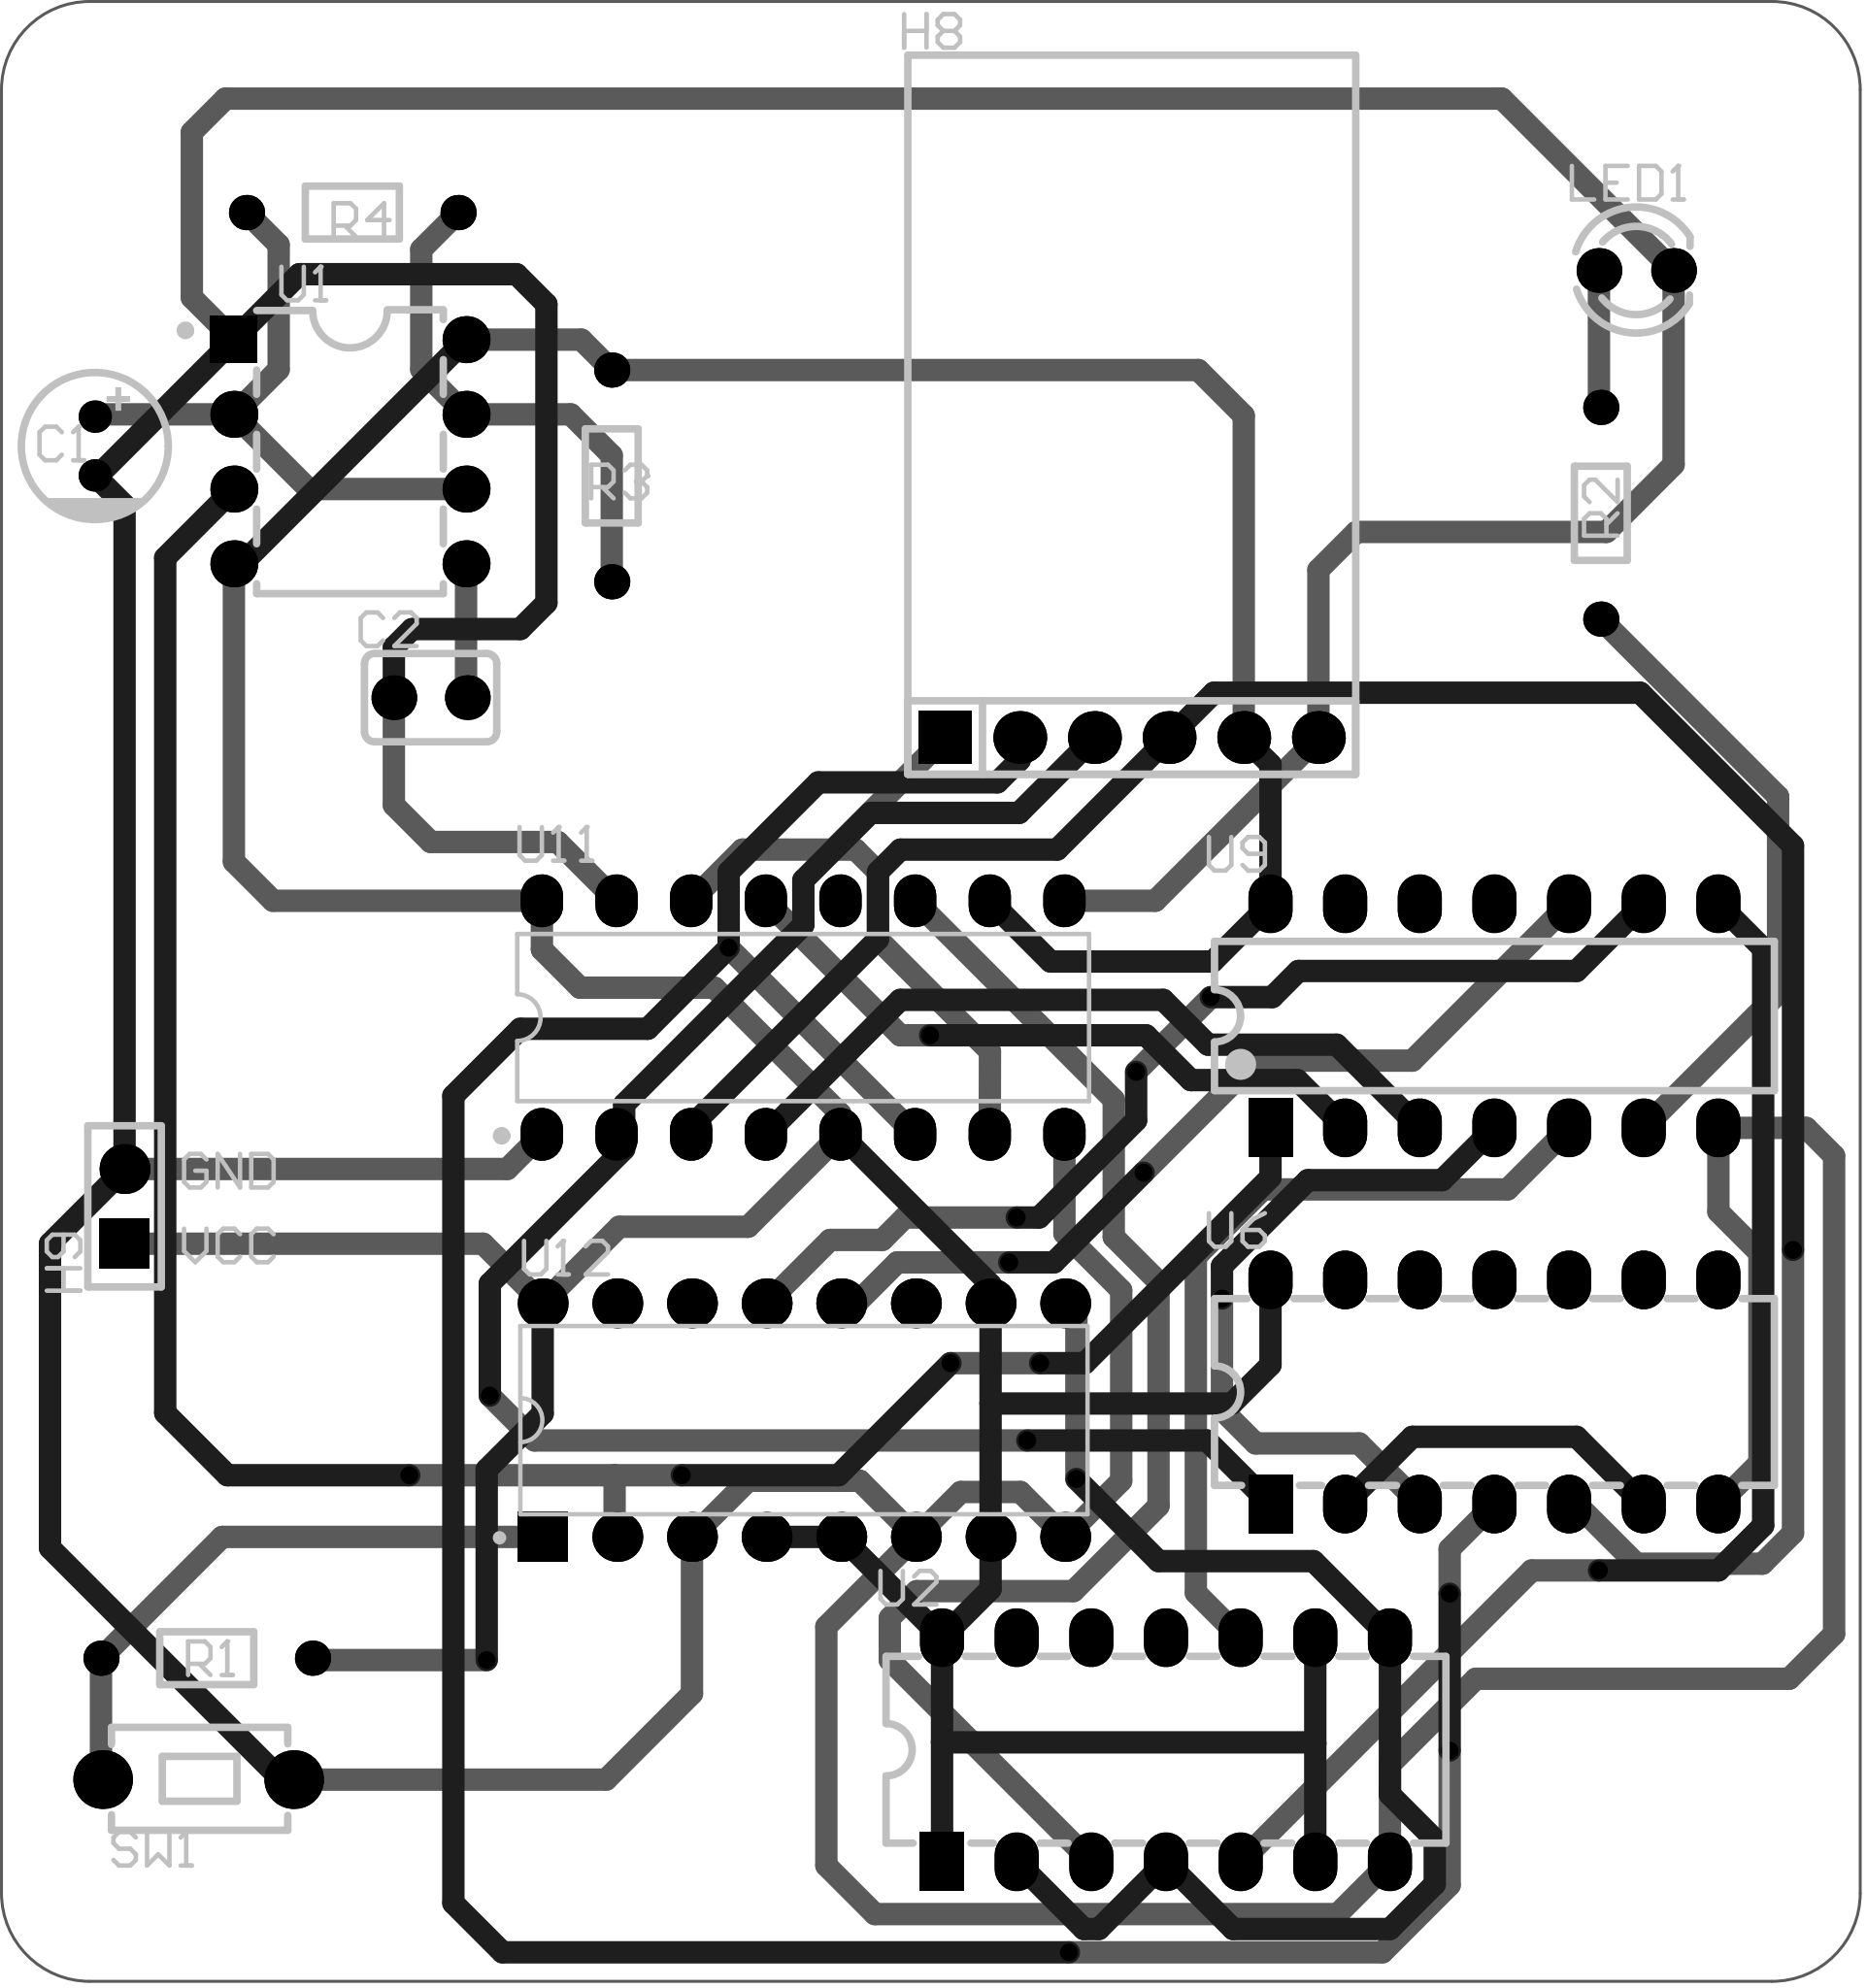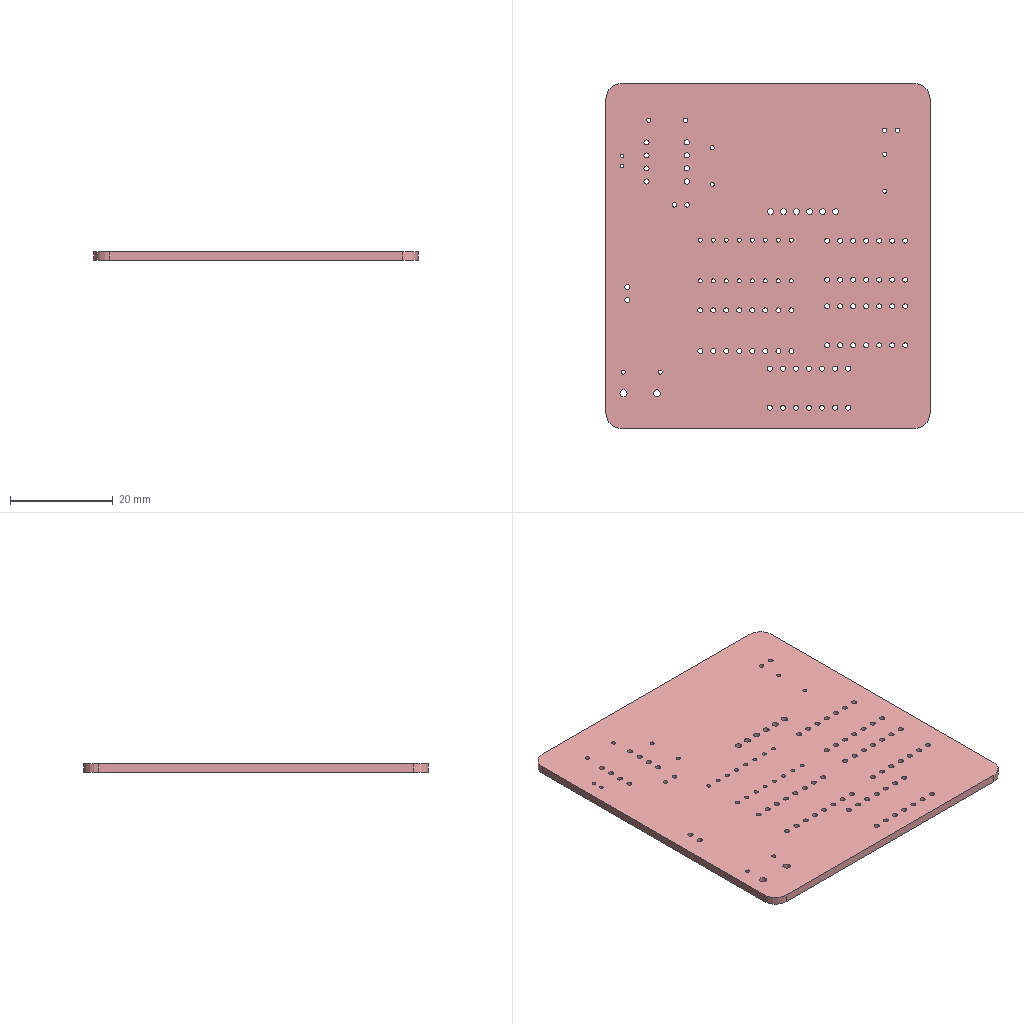Circuit board layout | Altium Designer | box 63.2 x 67.3 x 1.6 mm
Layer stack:
# Altium Designer layer stack of  (unit mm; dielectric type: 0 none, 1 core, 2 prepreg, 3 surface material)
index,name,kind,layer,copper_thickness_mm,dielectric_type,dielectric_thickness_mm,dielectric_material,dielectric_constant
0,Top Paste Mask Layer,other,,,,,,
1,Top Silkscreen Layer,other,,,,,,
2,Top Solder Mask Layer,dielectric,,,3,0.01,,3.3
3,Top Layer,copper,Top Layer,0.035,,,,
4,Dielectric1,dielectric,,,3,1.51,FR4,4.5
5,Bottom Layer,copper,Bottom Layer,0.035,,,,
6,Bottom Solder Mask Layer,dielectric,,,3,0.01,,3.3
7,Bottom Silkscreen Layer,other,,,,,,
8,Bottom Paste Mask Layer,other,,,,,,
# drill layer pairs: low layer,high layer
drill_pair,Top Layer,Bottom Layer
Part placement:
Designator,Comment,Layer,Footprint,Center-X(mm),Center-Y(mm),Rotation
R2,300Ω,TopLayer,Res_1/8W,130.619,126.111,270
H8,,TopLayer,HDR-TH_6P-P2.54-V-M-1,114.66,118.486,0
U1,NE555PE4,TopLayer,PDIP-8_L9.6-W6.4-P2.54-LS7.9-BL-1,88.058,128.204,270
C1,10uF,TopLayer,CAP-TH_BD5.0-P2.00-D0.5-FD,79.375,128.397,270
R3,47kΩ,TopLayer,Res_1/8W,96.965,127.381,90
R4,47kΩ,TopLayer,Res_1/8W,88.138,136.334,0
C2,100nF,TopLayer,CAP-TH_L4.5-W3.0-P2.50-D0.5,90.802,119.843,0
U11,74LS192D,TopLayer,PDIP-16_L19.3-W6.4-P2.54-LS7.94-BL,103.478,108.966,0
H9,,TopLayer,HDR-TH_2P-P2.54-V-F,80.388,102.548,90
LED1,,TopLayer,LED_TH-3mm,131.826,134.366,0
R1,10kΩ,TopLayer,Res_1/8W,83.185,87.186,180
SW1,,TopLayer,Key_TH_3.5x6x4.3,82.893,83.058,180
U2,SN74HC266N,TopLayer,PDIP-14_L19.3-W6.4-P2.54-LS7.6-BL,115.824,84.074,0
U6,CD74HC32EG4,TopLayer,PDIP-14_L19.3-W6.4-P2.54-LS7.6-BL,127,96.237,0
U9,74HC08DN,TopLayer,PDIP-14_L19.3-W6.5-P2.54-LS7.6-BL,127,109.026,0
U12,SN74HC161NG4,TopLayer,PDIP-16_L19.3-W6.4-P2.54-LS7.9-BL,103.505,95.279,0
Pad and via stacks:
# Altium Designer via and pad stacks of  (unit mm). Each distinct definition once, with the count of objects using it.
# via: kind,start_layer,end_layer,hole_mm,diameter_mm,mode(0 simple;1 top-mid-bottom;2 full stack),diameter_per_layer,count,example_net
# pad: kind,layer,hole_mm,hole_type(0 round;1 square;2 slot),plating,top_size,top_shape(1 round;2 rect;3 octagon;9 rounded rect),mid_size,bottom_size,mode,footprint,size_per_layer,count,example
pad,Multi-Layer,0.8001,0,plated,1.199x1.199,1,1.199x1.199,1.199x1.199,0,Res_1/8W,,8,R2.1
pad,Multi-Layer,1.2,0,plated,1.8x1.8,1,1.8x1.8,1.8x1.8,0,HDR-TH_6P-P2.54-V-M-1,,5,H8.6
pad,Multi-Layer,1.2,0,plated,1.8x1.8,2,1.8x1.8,1.8x1.8,0,HDR-TH_6P-P2.54-V-M-1,,1,H8.1
pad,Multi-Layer,1,0,plated,1.6x1.6,1,1.6x1.6,1.6x1.6,0,PDIP-8_L9.6-W6.4-P2.54-LS7.9-BL-1,,7,U1.8
pad,Multi-Layer,1,0,plated,1.6x1.6,2,1.6x1.6,1.6x1.6,0,PDIP-8_L9.6-W6.4-P2.54-LS7.9-BL-1,,1,U1.1
pad,Multi-Layer,0.7,0,plated,1.1x1.1,1,1.1x1.1,1.1x1.1,0,CAP-TH_BD5.0-P2.00-D0.5-FD,,2,C1.1
pad,Multi-Layer,0.9144,0,plated,1.524x1.524,1,1.524x1.524,1.524x1.524,0,CAP-TH_L4.5-W3.0-P2.50-D0.5,,2,C2.1
pad,Multi-Layer,0.8,0,plated,1.44x1.8,1,1.44x1.8,1.44x1.8,0,PDIP-16_L19.3-W6.4-P2.54-LS7.94-BL,,16,U11.1
pad,Multi-Layer,1,0,plated,1.7x1.7,2,1.7x1.7,1.7x1.7,0,HDR-TH_2P-P2.54-V-F,,1,H9.1
pad,Multi-Layer,1,0,plated,1.7x1.7,1,1.7x1.7,1.7x1.7,0,HDR-TH_2P-P2.54-V-F,,1,H9.2
pad,Multi-Layer,0.9144,0,plated,1.524x1.524,1,1.524x1.524,1.524x1.524,0,LED_TH-3mm,,2,LED1.1
pad,Multi-Layer,1.399,0,plated,1.999x1.999,1,1.999x1.999,1.999x1.999,0,Key_TH_3.5x6x4.3,,2,SW1.A
pad,Multi-Layer,1,0,plated,1.5x2,2,1.5x2,1.5x2,0,PDIP-14_L19.3-W6.4-P2.54-LS7.6-BL,,2,U2.1
pad,Multi-Layer,1,0,plated,1.5x2,1,1.5x2,1.5x2,0,PDIP-14_L19.3-W6.4-P2.54-LS7.6-BL,,26,U2.2
pad,Multi-Layer,1,0,plated,1.5x2,1,1.5x2,1.5x2,0,PDIP-14_L19.3-W6.5-P2.54-LS7.6-BL,,13,U9.8
pad,Multi-Layer,1,0,plated,1.5x2,2,1.5x2,1.5x2,0,PDIP-14_L19.3-W6.5-P2.54-LS7.6-BL,,1,U9.1
pad,Multi-Layer,1,0,plated,1.7x1.7,2,1.7x1.7,1.7x1.7,0,PDIP-16_L19.3-W6.4-P2.54-LS7.9-BL,,1,U12.1
pad,Multi-Layer,1,0,plated,1.7x1.7,1,1.7x1.7,1.7x1.7,0,PDIP-16_L19.3-W6.4-P2.54-LS7.9-BL,,15,U12.2
via,Top Layer,Bottom Layer,0.3048,0.6096,0,,20,DCDB
via,Top Layer,Bottom Layer,0.3048,0.61,0,,1,VCC
Design rules, without the lines most boards share:
# Altium Designer design rules of  (exported by Altium Designer, unit mm)
# columns: name | kind | enabled | priority | scope1 | scope2 | descriptor | typed fields (field=value)
copperThickness2oz | 0 | disabled | 1 | All | All | Clearance Constraint (Gap=6mil) (Disabled)(All),(All) | gap=0.1524
Plane_innerPlane | 0 | disabled | 2 | All | All | Clearance Constraint (Gap=6mil) (Disabled)(All),(All) | gap=0.1524
Copper_copperRegion | 0 | disabled | 3 | All | All | Clearance Constraint (Gap=6mil) (Disabled)(All),(All) | gap=0.1524
copperThickness1oz | 0 | enabled | 4 | All | All | Clearance Constraint (Gap=6mil) (All),(All) | gap=0.1524
otherClearance | 52 | enabled | 1 | All | All | Hole To Hole Clearance (Gap=11.8mil) (All),(All) | gap=0.2997
copperThickness1oz_2 | 2 | enabled | 2 | All | All | Width Constraint (Min=5mil) (Max=100mil) (Preferred=30mil) (All) |
viaSize | 11 | enabled | 1 | All | All | Routing Via (MinHoleWidth=11.8mil) (MaxHoleWidth=248mil) (PreferredHoleWidth=12mil) (MinWidth=19.7mil) (MaxWidth=393.7mil) (PreferedWidth=24mil) (All) | via_min_hole=0.2997 via_max_hole=6.299 via_preferred_diameter=0.6096 via_preferred_hole=0.3048